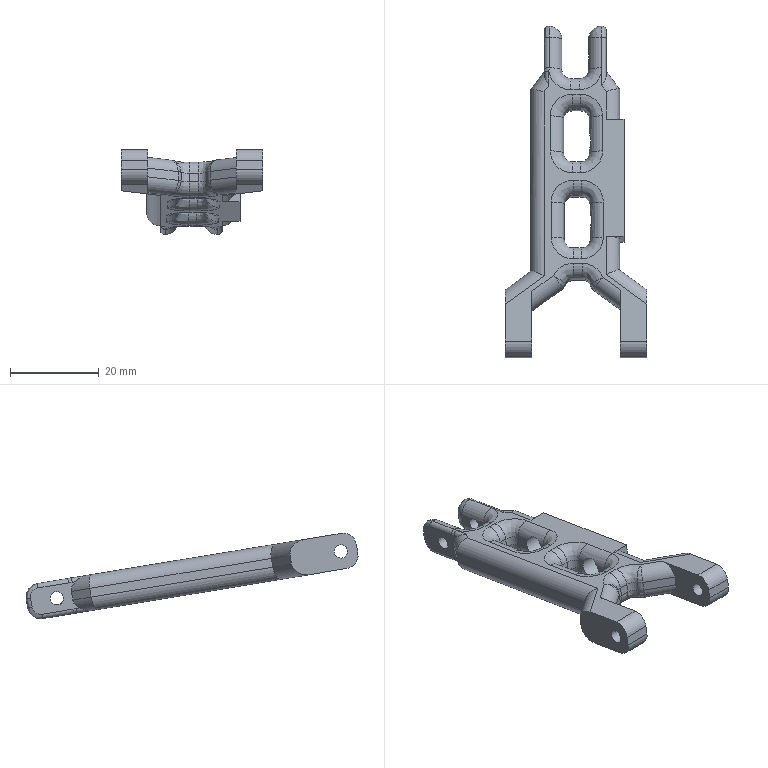Part | STEP file | Wytnij-wyci_gni_cie2_2 | 1 solid | 155 faces | box 32 x 74.835 x 19.276 mm | volume 7840 mm3 | cylinder 78 | plane 39 | spline 38 | commonest cylinder face diameters 6 x48 4 x14 2 x9 3 x4 5.05 x3